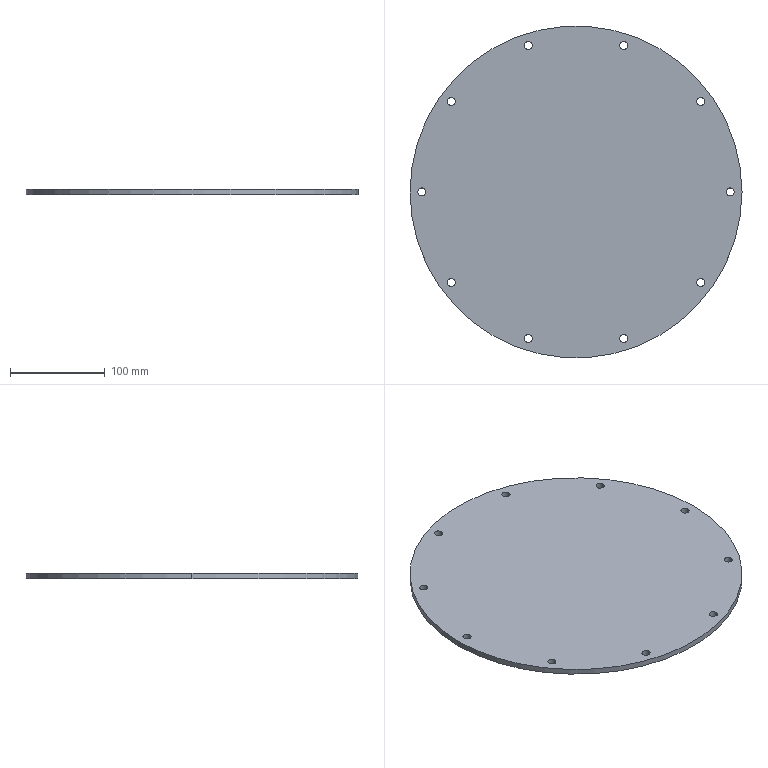Part | SolidWorks | features BaseBody 1 | 1 solid | 24 faces | box 350 x 350 x 6 mm | volume 573863 mm3 | cylinder 22 | plane 2 | commonest cylinder face diameters 8.5 x20 350 x2
STEP:
#1=CARTESIAN_POINT('',(127.215,95.515,-6.));
#2=VERTEX_POINT('',#1);
#3=CARTESIAN_POINT('',(135.715,95.515,-6.));
#4=VERTEX_POINT('',#3);
#5=CARTESIAN_POINT('',(131.465,95.515,-6.));
#6=DIRECTION('',(0.,0.,1.));
#7=DIRECTION('',(1.,0.,0.));
#8=AXIS2_PLACEMENT_3D('',#5,#6,#7);
#9=CIRCLE('',#8,4.25);
#10=EDGE_CURVE('',#2,#4,#9,.T.);
#11=ORIENTED_EDGE('',*,*,#10,.F.);
#12=CARTESIAN_POINT('',(127.215,95.515,0.));
#13=VERTEX_POINT('',#12);
#14=CARTESIAN_POINT('',(127.215,95.515,-20.));
#15=DIRECTION('',(0.,0.,1.));
#16=VECTOR('',#15,1000.);
#17=LINE('',#14,#16);
#18=EDGE_CURVE('',#2,#13,#17,.T.);
#19=ORIENTED_EDGE('',*,*,#18,.T.);
#20=CARTESIAN_POINT('',(135.715,95.515,0.));
#21=VERTEX_POINT('',#20);
#22=CARTESIAN_POINT('',(131.465,95.515,0.));
#23=DIRECTION('',(0.,0.,1.));
#24=DIRECTION('',(0.809,0.5878,0.));
#25=AXIS2_PLACEMENT_3D('',#22,#23,#24);
#26=CIRCLE('',#25,4.25);
#27=EDGE_CURVE('',#13,#21,#26,.T.);
#28=ORIENTED_EDGE('',*,*,#27,.T.);
#29=CARTESIAN_POINT('',(135.715,95.515,-20.));
#30=DIRECTION('',(0.,0.,1.));
#31=VECTOR('',#30,1000.);
#32=LINE('',#29,#31);
#33=EDGE_CURVE('',#4,#21,#32,.T.);
#34=ORIENTED_EDGE('',*,*,#33,.F.);
#35=EDGE_LOOP('',(#11,#19,#28,#34));
#36=FACE_OUTER_BOUND('',#35,.T.);
#37=CARTESIAN_POINT('',(131.465,95.515,-20.));
#38=DIRECTION('',(0.,0.,1.));
#39=DIRECTION('',(1.,0.,0.));
#40=AXIS2_PLACEMENT_3D('',#37,#38,#39);
#41=CYLINDRICAL_SURFACE('',#40,4.25);
#42=ADVANCED_FACE('',(#36),#41,.F.);
#43=CARTESIAN_POINT('',(45.965,154.547,-6.));
#44=VERTEX_POINT('',#43);
#45=CARTESIAN_POINT('',(54.465,154.547,-6.));
#46=VERTEX_POINT('',#45);
#47=CARTESIAN_POINT('',(50.215,154.547,-6.));
#48=DIRECTION('',(0.,0.,1.));
#49=DIRECTION('',(1.,0.,0.));
#50=AXIS2_PLACEMENT_3D('',#47,#48,#49);
#51=CIRCLE('',#50,4.25);
#52=EDGE_CURVE('',#44,#46,#51,.T.);
#53=ORIENTED_EDGE('',*,*,#52,.F.);
#54=CARTESIAN_POINT('',(45.965,154.547,0.));
#55=VERTEX_POINT('',#54);
#56=CARTESIAN_POINT('',(45.965,154.547,-20.));
#57=DIRECTION('',(0.,0.,1.));
#58=VECTOR('',#57,1000.);
#59=LINE('',#56,#58);
#60=EDGE_CURVE('',#44,#55,#59,.T.);
#61=ORIENTED_EDGE('',*,*,#60,.T.);
#62=CARTESIAN_POINT('',(54.465,154.547,0.));
#63=VERTEX_POINT('',#62);
#64=CARTESIAN_POINT('',(50.215,154.547,0.));
#65=DIRECTION('',(0.,0.,1.));
#66=DIRECTION('',(0.309,0.9511,0.));
#67=AXIS2_PLACEMENT_3D('',#64,#65,#66);
#68=CIRCLE('',#67,4.25);
#69=EDGE_CURVE('',#55,#63,#68,.T.);
#70=ORIENTED_EDGE('',*,*,#69,.T.);
#71=CARTESIAN_POINT('',(54.465,154.547,-20.));
#72=DIRECTION('',(0.,0.,1.));
#73=VECTOR('',#72,1000.);
#74=LINE('',#71,#73);
#75=EDGE_CURVE('',#46,#63,#74,.T.);
#76=ORIENTED_EDGE('',*,*,#75,.F.);
#77=EDGE_LOOP('',(#53,#61,#70,#76));
#78=FACE_OUTER_BOUND('',#77,.T.);
#79=CARTESIAN_POINT('',(50.215,154.547,-20.));
#80=DIRECTION('',(0.,0.,1.));
#81=DIRECTION('',(1.,0.,0.));
#82=AXIS2_PLACEMENT_3D('',#79,#80,#81);
#83=CYLINDRICAL_SURFACE('',#82,4.25);
#84=ADVANCED_FACE('',(#78),#83,.F.);
#85=CARTESIAN_POINT('',(-54.465,154.547,-6.));
#86=VERTEX_POINT('',#85);
#87=CARTESIAN_POINT('',(-45.965,154.547,-6.));
#88=VERTEX_POINT('',#87);
#89=CARTESIAN_POINT('',(-50.215,154.547,-6.));
#90=DIRECTION('',(0.,0.,1.));
#91=DIRECTION('',(1.,0.,0.));
#92=AXIS2_PLACEMENT_3D('',#89,#90,#91);
#93=CIRCLE('',#92,4.25);
#94=EDGE_CURVE('',#86,#88,#93,.T.);
#95=ORIENTED_EDGE('',*,*,#94,.F.);
#96=CARTESIAN_POINT('',(-54.465,154.547,0.));
#97=VERTEX_POINT('',#96);
#98=CARTESIAN_POINT('',(-54.465,154.547,-20.));
#99=DIRECTION('',(0.,0.,1.));
#100=VECTOR('',#99,1000.);
#101=LINE('',#98,#100);
#102=EDGE_CURVE('',#86,#97,#101,.T.);
#103=ORIENTED_EDGE('',*,*,#102,.T.);
#104=CARTESIAN_POINT('',(-45.965,154.547,0.));
#105=VERTEX_POINT('',#104);
#106=CARTESIAN_POINT('',(-50.215,154.547,0.));
#107=DIRECTION('',(0.,0.,1.));
#108=DIRECTION('',(-0.309,0.9511,0.));
#109=AXIS2_PLACEMENT_3D('',#106,#107,#108);
#110=CIRCLE('',#109,4.25);
#111=EDGE_CURVE('',#97,#105,#110,.T.);
#112=ORIENTED_EDGE('',*,*,#111,.T.);
#113=CARTESIAN_POINT('',(-45.965,154.547,-20.));
#114=DIRECTION('',(0.,0.,1.));
#115=VECTOR('',#114,1000.);
#116=LINE('',#113,#115);
#117=EDGE_CURVE('',#88,#105,#116,.T.);
#118=ORIENTED_EDGE('',*,*,#117,.F.);
#119=EDGE_LOOP('',(#95,#103,#112,#118));
#120=FACE_OUTER_BOUND('',#119,.T.);
#121=CARTESIAN_POINT('',(-50.215,154.547,-20.));
#122=DIRECTION('',(0.,0.,1.));
#123=DIRECTION('',(1.,0.,0.));
#124=AXIS2_PLACEMENT_3D('',#121,#122,#123);
#125=CYLINDRICAL_SURFACE('',#124,4.25);
#126=ADVANCED_FACE('',(#120),#125,.F.);
#127=CARTESIAN_POINT('',(-135.715,95.515,-6.));
#128=VERTEX_POINT('',#127);
#129=CARTESIAN_POINT('',(-127.215,95.515,-6.));
#130=VERTEX_POINT('',#129);
#131=CARTESIAN_POINT('',(-131.465,95.515,-6.));
#132=DIRECTION('',(0.,0.,1.));
#133=DIRECTION('',(1.,0.,0.));
#134=AXIS2_PLACEMENT_3D('',#131,#132,#133);
#135=CIRCLE('',#134,4.25);
#136=EDGE_CURVE('',#128,#130,#135,.T.);
#137=ORIENTED_EDGE('',*,*,#136,.F.);
#138=CARTESIAN_POINT('',(-135.715,95.515,0.));
#139=VERTEX_POINT('',#138);
#140=CARTESIAN_POINT('',(-135.715,95.515,-20.));
#141=DIRECTION('',(0.,0.,1.));
#142=VECTOR('',#141,1000.);
#143=LINE('',#140,#142);
#144=EDGE_CURVE('',#128,#139,#143,.T.);
#145=ORIENTED_EDGE('',*,*,#144,.T.);
#146=CARTESIAN_POINT('',(-127.215,95.515,0.));
#147=VERTEX_POINT('',#146);
#148=CARTESIAN_POINT('',(-131.465,95.515,0.));
#149=DIRECTION('',(0.,0.,1.));
#150=DIRECTION('',(-0.809,0.5878,0.));
#151=AXIS2_PLACEMENT_3D('',#148,#149,#150);
#152=CIRCLE('',#151,4.25);
#153=EDGE_CURVE('',#139,#147,#152,.T.);
#154=ORIENTED_EDGE('',*,*,#153,.T.);
#155=CARTESIAN_POINT('',(-127.215,95.515,-20.));
#156=DIRECTION('',(0.,0.,1.));
#157=VECTOR('',#156,1000.);
#158=LINE('',#155,#157);
#159=EDGE_CURVE('',#130,#147,#158,.T.);
#160=ORIENTED_EDGE('',*,*,#159,.F.);
#161=EDGE_LOOP('',(#137,#145,#154,#160));
#162=FACE_OUTER_BOUND('',#161,.T.);
#163=CARTESIAN_POINT('',(-131.465,95.515,-20.));
#164=DIRECTION('',(0.,0.,1.));
#165=DIRECTION('',(1.,0.,0.));
#166=AXIS2_PLACEMENT_3D('',#163,#164,#165);
#167=CYLINDRICAL_SURFACE('',#166,4.25);
#168=ADVANCED_FACE('',(#162),#167,.F.);
#169=CARTESIAN_POINT('',(-166.75,0.,-6.));
#170=VERTEX_POINT('',#169);
#171=CARTESIAN_POINT('',(-158.25,0.,-6.));
#172=VERTEX_POINT('',#171);
#173=CARTESIAN_POINT('',(-162.5,0.,-6.));
#174=DIRECTION('',(0.,0.,1.));
#175=DIRECTION('',(1.,0.,0.));
#176=AXIS2_PLACEMENT_3D('',#173,#174,#175);
#177=CIRCLE('',#176,4.25);
#178=EDGE_CURVE('',#170,#172,#177,.T.);
#179=ORIENTED_EDGE('',*,*,#178,.F.);
#180=CARTESIAN_POINT('',(-166.75,0.,0.));
#181=VERTEX_POINT('',#180);
#182=CARTESIAN_POINT('',(-166.75,0.,-20.));
#183=DIRECTION('',(0.,0.,1.));
#184=VECTOR('',#183,1000.);
#185=LINE('',#182,#184);
#186=EDGE_CURVE('',#170,#181,#185,.T.);
#187=ORIENTED_EDGE('',*,*,#186,.T.);
#188=CARTESIAN_POINT('',(-158.25,0.,0.));
#189=VERTEX_POINT('',#188);
#190=CARTESIAN_POINT('',(-162.5,0.,0.));
#191=DIRECTION('',(0.,0.,1.));
#192=DIRECTION('',(-1.,0.,0.));
#193=AXIS2_PLACEMENT_3D('',#190,#191,#192);
#194=CIRCLE('',#193,4.25);
#195=EDGE_CURVE('',#181,#189,#194,.T.);
#196=ORIENTED_EDGE('',*,*,#195,.T.);
#197=CARTESIAN_POINT('',(-158.25,0.,-20.));
#198=DIRECTION('',(0.,0.,1.));
#199=VECTOR('',#198,1000.);
#200=LINE('',#197,#199);
#201=EDGE_CURVE('',#172,#189,#200,.T.);
#202=ORIENTED_EDGE('',*,*,#201,.F.);
#203=EDGE_LOOP('',(#179,#187,#196,#202));
#204=FACE_OUTER_BOUND('',#203,.T.);
#205=CARTESIAN_POINT('',(-162.5,0.,-20.));
#206=DIRECTION('',(0.,0.,1.));
#207=DIRECTION('',(1.,0.,0.));
#208=AXIS2_PLACEMENT_3D('',#205,#206,#207);
#209=CYLINDRICAL_SURFACE('',#208,4.25);
#210=ADVANCED_FACE('',(#204),#209,.F.);
#211=CARTESIAN_POINT('',(-135.715,-95.515,-6.));
#212=VERTEX_POINT('',#211);
#213=CARTESIAN_POINT('',(-127.215,-95.515,-6.));
#214=VERTEX_POINT('',#213);
#215=CARTESIAN_POINT('',(-131.465,-95.515,-6.));
#216=DIRECTION('',(0.,0.,1.));
#217=DIRECTION('',(1.,0.,0.));
#218=AXIS2_PLACEMENT_3D('',#215,#216,#217);
#219=CIRCLE('',#218,4.25);
#220=EDGE_CURVE('',#212,#214,#219,.T.);
#221=ORIENTED_EDGE('',*,*,#220,.F.);
#222=CARTESIAN_POINT('',(-135.715,-95.515,0.));
#223=VERTEX_POINT('',#222);
#224=CARTESIAN_POINT('',(-135.715,-95.515,-20.));
#225=DIRECTION('',(0.,0.,1.));
#226=VECTOR('',#225,1000.);
#227=LINE('',#224,#226);
#228=EDGE_CURVE('',#212,#223,#227,.T.);
#229=ORIENTED_EDGE('',*,*,#228,.T.);
#230=CARTESIAN_POINT('',(-127.215,-95.515,0.));
#231=VERTEX_POINT('',#230);
#232=CARTESIAN_POINT('',(-131.465,-95.515,0.));
#233=DIRECTION('',(0.,0.,1.));
#234=DIRECTION('',(-0.809,-0.5878,0.));
#235=AXIS2_PLACEMENT_3D('',#232,#233,#234);
#236=CIRCLE('',#235,4.25);
#237=EDGE_CURVE('',#223,#231,#236,.T.);
#238=ORIENTED_EDGE('',*,*,#237,.T.);
#239=CARTESIAN_POINT('',(-127.215,-95.515,-20.));
#240=DIRECTION('',(0.,0.,1.));
#241=VECTOR('',#240,1000.);
#242=LINE('',#239,#241);
#243=EDGE_CURVE('',#214,#231,#242,.T.);
#244=ORIENTED_EDGE('',*,*,#243,.F.);
#245=EDGE_LOOP('',(#221,#229,#238,#244));
#246=FACE_OUTER_BOUND('',#245,.T.);
#247=CARTESIAN_POINT('',(-131.465,-95.515,-20.));
#248=DIRECTION('',(0.,0.,1.));
#249=DIRECTION('',(1.,0.,0.));
#250=AXIS2_PLACEMENT_3D('',#247,#248,#249);
#251=CYLINDRICAL_SURFACE('',#250,4.25);
#252=ADVANCED_FACE('',(#246),#251,.F.);
#253=CARTESIAN_POINT('',(-54.465,-154.547,-6.));
#254=VERTEX_POINT('',#253);
#255=CARTESIAN_POINT('',(-45.965,-154.547,-6.));
#256=VERTEX_POINT('',#255);
#257=CARTESIAN_POINT('',(-50.215,-154.547,-6.));
#258=DIRECTION('',(0.,0.,1.));
#259=DIRECTION('',(1.,0.,0.));
#260=AXIS2_PLACEMENT_3D('',#257,#258,#259);
#261=CIRCLE('',#260,4.25);
#262=EDGE_CURVE('',#254,#256,#261,.T.);
#263=ORIENTED_EDGE('',*,*,#262,.F.);
#264=CARTESIAN_POINT('',(-54.465,-154.547,0.));
#265=VERTEX_POINT('',#264);
#266=CARTESIAN_POINT('',(-54.465,-154.547,-20.));
#267=DIRECTION('',(0.,0.,1.));
#268=VECTOR('',#267,1000.);
#269=LINE('',#266,#268);
#270=EDGE_CURVE('',#254,#265,#269,.T.);
#271=ORIENTED_EDGE('',*,*,#270,.T.);
#272=CARTESIAN_POINT('',(-45.965,-154.547,0.));
#273=VERTEX_POINT('',#272);
#274=CARTESIAN_POINT('',(-50.215,-154.547,0.));
#275=DIRECTION('',(0.,0.,1.));
#276=DIRECTION('',(-0.309,-0.9511,0.));
#277=AXIS2_PLACEMENT_3D('',#274,#275,#276);
#278=CIRCLE('',#277,4.25);
#279=EDGE_CURVE('',#265,#273,#278,.T.);
#280=ORIENTED_EDGE('',*,*,#279,.T.);
#281=CARTESIAN_POINT('',(-45.965,-154.547,-20.));
#282=DIRECTION('',(0.,0.,1.));
#283=VECTOR('',#282,1000.);
#284=LINE('',#281,#283);
#285=EDGE_CURVE('',#256,#273,#284,.T.);
#286=ORIENTED_EDGE('',*,*,#285,.F.);
#287=EDGE_LOOP('',(#263,#271,#280,#286));
#288=FACE_OUTER_BOUND('',#287,.T.);
#289=CARTESIAN_POINT('',(-50.215,-154.547,-20.));
#290=DIRECTION('',(0.,0.,1.));
#291=DIRECTION('',(1.,0.,0.));
#292=AXIS2_PLACEMENT_3D('',#289,#290,#291);
#293=CYLINDRICAL_SURFACE('',#292,4.25);
#294=ADVANCED_FACE('',(#288),#293,.F.);
#295=CARTESIAN_POINT('',(45.965,-154.547,-6.));
#296=VERTEX_POINT('',#295);
#297=CARTESIAN_POINT('',(54.465,-154.547,-6.));
#298=VERTEX_POINT('',#297);
#299=CARTESIAN_POINT('',(50.215,-154.547,-6.));
#300=DIRECTION('',(0.,0.,1.));
#301=DIRECTION('',(1.,0.,0.));
#302=AXIS2_PLACEMENT_3D('',#299,#300,#301);
#303=CIRCLE('',#302,4.25);
#304=EDGE_CURVE('',#296,#298,#303,.T.);
#305=ORIENTED_EDGE('',*,*,#304,.F.);
#306=CARTESIAN_POINT('',(45.965,-154.547,0.));
#307=VERTEX_POINT('',#306);
#308=CARTESIAN_POINT('',(45.965,-154.547,-20.));
#309=DIRECTION('',(0.,0.,1.));
#310=VECTOR('',#309,1000.);
#311=LINE('',#308,#310);
#312=EDGE_CURVE('',#296,#307,#311,.T.);
#313=ORIENTED_EDGE('',*,*,#312,.T.);
#314=CARTESIAN_POINT('',(54.465,-154.547,0.));
#315=VERTEX_POINT('',#314);
#316=CARTESIAN_POINT('',(50.215,-154.547,0.));
#317=DIRECTION('',(0.,0.,1.));
#318=DIRECTION('',(0.309,-0.9511,0.));
#319=AXIS2_PLACEMENT_3D('',#316,#317,#318);
#320=CIRCLE('',#319,4.25);
#321=EDGE_CURVE('',#307,#315,#320,.T.);
#322=ORIENTED_EDGE('',*,*,#321,.T.);
#323=CARTESIAN_POINT('',(54.465,-154.547,-20.));
#324=DIRECTION('',(0.,0.,1.));
#325=VECTOR('',#324,1000.);
#326=LINE('',#323,#325);
#327=EDGE_CURVE('',#298,#315,#326,.T.);
#328=ORIENTED_EDGE('',*,*,#327,.F.);
#329=EDGE_LOOP('',(#305,#313,#322,#328));
#330=FACE_OUTER_BOUND('',#329,.T.);
#331=CARTESIAN_POINT('',(50.215,-154.547,-20.));
#332=DIRECTION('',(0.,0.,1.));
#333=DIRECTION('',(1.,0.,0.));
#334=AXIS2_PLACEMENT_3D('',#331,#332,#333);
#335=CYLINDRICAL_SURFACE('',#334,4.25);
#336=ADVANCED_FACE('',(#330),#335,.F.);
#337=CARTESIAN_POINT('',(127.215,-95.515,-6.));
#338=VERTEX_POINT('',#337);
#339=CARTESIAN_POINT('',(135.715,-95.515,-6.));
#340=VERTEX_POINT('',#339);
#341=CARTESIAN_POINT('',(131.465,-95.515,-6.));
#342=DIRECTION('',(0.,0.,1.));
#343=DIRECTION('',(1.,0.,0.));
#344=AXIS2_PLACEMENT_3D('',#341,#342,#343);
#345=CIRCLE('',#344,4.25);
#346=EDGE_CURVE('',#338,#340,#345,.T.);
#347=ORIENTED_EDGE('',*,*,#346,.F.);
#348=CARTESIAN_POINT('',(127.215,-95.515,0.));
#349=VERTEX_POINT('',#348);
#350=CARTESIAN_POINT('',(127.215,-95.515,-20.));
#351=DIRECTION('',(0.,0.,1.));
#352=VECTOR('',#351,1000.);
#353=LINE('',#350,#352);
#354=EDGE_CURVE('',#338,#349,#353,.T.);
#355=ORIENTED_EDGE('',*,*,#354,.T.);
#356=CARTESIAN_POINT('',(135.715,-95.515,0.));
#357=VERTEX_POINT('',#356);
#358=CARTESIAN_POINT('',(131.465,-95.515,0.));
#359=DIRECTION('',(0.,0.,1.));
#360=DIRECTION('',(0.809,-0.5878,0.));
#361=AXIS2_PLACEMENT_3D('',#358,#359,#360);
#362=CIRCLE('',#361,4.25);
#363=EDGE_CURVE('',#349,#357,#362,.T.);
#364=ORIENTED_EDGE('',*,*,#363,.T.);
#365=CARTESIAN_POINT('',(135.715,-95.515,-20.));
#366=DIRECTION('',(0.,0.,1.));
#367=VECTOR('',#366,1000.);
#368=LINE('',#365,#367);
#369=EDGE_CURVE('',#340,#357,#368,.T.);
#370=ORIENTED_EDGE('',*,*,#369,.F.);
#371=EDGE_LOOP('',(#347,#355,#364,#370));
#372=FACE_OUTER_BOUND('',#371,.T.);
#373=CARTESIAN_POINT('',(131.465,-95.515,-20.));
#374=DIRECTION('',(0.,0.,1.));
#375=DIRECTION('',(1.,0.,0.));
#376=AXIS2_PLACEMENT_3D('',#373,#374,#375);
#377=CYLINDRICAL_SURFACE('',#376,4.25);
#378=ADVANCED_FACE('',(#372),#377,.F.);
#379=CARTESIAN_POINT('',(158.25,0.,-6.));
#380=VERTEX_POINT('',#379);
#381=CARTESIAN_POINT('',(166.75,0.,-6.));
#382=VERTEX_POINT('',#381);
#383=CARTESIAN_POINT('',(162.5,0.,-6.));
#384=DIRECTION('',(0.,0.,1.));
#385=DIRECTION('',(1.,0.,0.));
#386=AXIS2_PLACEMENT_3D('',#383,#384,#385);
#387=CIRCLE('',#386,4.25);
#388=EDGE_CURVE('',#380,#382,#387,.T.);
#389=ORIENTED_EDGE('',*,*,#388,.F.);
#390=CARTESIAN_POINT('',(158.25,0.,0.));
#391=VERTEX_POINT('',#390);
#392=CARTESIAN_POINT('',(158.25,0.,-20.));
#393=DIRECTION('',(0.,0.,1.));
#394=VECTOR('',#393,1000.);
#395=LINE('',#392,#394);
#396=EDGE_CURVE('',#380,#391,#395,.T.);
#397=ORIENTED_EDGE('',*,*,#396,.T.);
#398=CARTESIAN_POINT('',(166.75,0.,0.));
#399=VERTEX_POINT('',#398);
#400=CARTESIAN_POINT('',(162.5,0.,0.));
#401=DIRECTION('',(0.,0.,1.));
#402=DIRECTION('',(1.,0.,0.));
#403=AXIS2_PLACEMENT_3D('',#400,#401,#402);
#404=CIRCLE('',#403,4.25);
#405=EDGE_CURVE('',#391,#399,#404,.T.);
#406=ORIENTED_EDGE('',*,*,#405,.T.);
#407=CARTESIAN_POINT('',(166.75,0.,-20.));
#408=DIRECTION('',(0.,0.,1.));
#409=VECTOR('',#408,1000.);
#410=LINE('',#407,#409);
#411=EDGE_CURVE('',#382,#399,#410,.T.);
#412=ORIENTED_EDGE('',*,*,#411,.F.);
#413=EDGE_LOOP('',(#389,#397,#406,#412));
#414=FACE_OUTER_BOUND('',#413,.T.);
#415=CARTESIAN_POINT('',(162.5,0.,-20.));
#416=DIRECTION('',(0.,0.,1.));
#417=DIRECTION('',(1.,0.,0.));
#418=AXIS2_PLACEMENT_3D('',#415,#416,#417);
#419=CYLINDRICAL_SURFACE('',#418,4.25);
#420=ADVANCED_FACE('',(#414),#419,.F.);
#421=CARTESIAN_POINT('',(175.,0.,-6.));
#422=VERTEX_POINT('',#421);
#423=CARTESIAN_POINT('',(-175.,0.,-6.));
#424=VERTEX_POINT('',#423);
#425=CARTESIAN_POINT('',(0.,0.,-6.));
#426=DIRECTION('',(0.,0.,1.));
#427=DIRECTION('',(1.,0.,0.));
#428=AXIS2_PLACEMENT_3D('',#425,#426,#427);
#429=CIRCLE('',#428,175.);
#430=EDGE_CURVE('',#422,#424,#429,.T.);
#431=ORIENTED_EDGE('',*,*,#430,.T.);
#432=CARTESIAN_POINT('',(-175.,0.,0.));
#433=VERTEX_POINT('',#432);
#434=CARTESIAN_POINT('',(-175.,0.,-6.));
#435=DIRECTION('',(0.,0.,1.));
#436=VECTOR('',#435,1000.);
#437=LINE('',#434,#436);
#438=EDGE_CURVE('',#424,#433,#437,.T.);
#439=ORIENTED_EDGE('',*,*,#438,.T.);
#440=CARTESIAN_POINT('',(175.,0.,0.));
#441=VERTEX_POINT('',#440);
#442=CARTESIAN_POINT('',(0.,0.,0.));
#443=DIRECTION('',(0.,0.,1.));
#444=DIRECTION('',(1.,0.,0.));
#445=AXIS2_PLACEMENT_3D('',#442,#443,#444);
#446=CIRCLE('',#445,175.);
#447=EDGE_CURVE('',#441,#433,#446,.T.);
#448=ORIENTED_EDGE('',*,*,#447,.F.);
#449=CARTESIAN_POINT('',(175.,0.,-6.));
#450=DIRECTION('',(0.,0.,1.));
#451=VECTOR('',#450,1000.);
#452=LINE('',#449,#451);
#453=EDGE_CURVE('',#422,#441,#452,.T.);
#454=ORIENTED_EDGE('',*,*,#453,.F.);
#455=EDGE_LOOP('',(#431,#439,#448,#454));
#456=FACE_OUTER_BOUND('',#455,.T.);
#457=CARTESIAN_POINT('',(0.,0.,-6.));
#458=DIRECTION('',(0.,0.,1.));
#459=DIRECTION('',(1.,0.,0.));
#460=AXIS2_PLACEMENT_3D('',#457,#458,#459);
#461=CYLINDRICAL_SURFACE('',#460,175.);
#462=ADVANCED_FACE('',(#456),#461,.T.);
#463=ORIENTED_EDGE('',*,*,#438,.F.);
#464=CARTESIAN_POINT('',(0.,0.,-6.));
#465=DIRECTION('',(0.,0.,1.));
#466=DIRECTION('',(1.,0.,0.));
#467=AXIS2_PLACEMENT_3D('',#464,#465,#466);
#468=CIRCLE('',#467,175.);
#469=EDGE_CURVE('',#424,#422,#468,.T.);
#470=ORIENTED_EDGE('',*,*,#469,.T.);
#471=ORIENTED_EDGE('',*,*,#453,.T.);
#472=CARTESIAN_POINT('',(0.,0.,0.));
#473=DIRECTION('',(0.,0.,1.));
#474=DIRECTION('',(1.,0.,0.));
#475=AXIS2_PLACEMENT_3D('',#472,#473,#474);
#476=CIRCLE('',#475,175.);
#477=EDGE_CURVE('',#433,#441,#476,.T.);
#478=ORIENTED_EDGE('',*,*,#477,.F.);
#479=EDGE_LOOP('',(#463,#470,#471,#478));
#480=FACE_OUTER_BOUND('',#479,.T.);
#481=CARTESIAN_POINT('',(0.,0.,-6.));
#482=DIRECTION('',(0.,0.,1.));
#483=DIRECTION('',(1.,0.,0.));
#484=AXIS2_PLACEMENT_3D('',#481,#482,#483);
#485=CYLINDRICAL_SURFACE('',#484,175.);
#486=ADVANCED_FACE('',(#480),#485,.T.);
#487=ORIENTED_EDGE('',*,*,#430,.F.);
#488=ORIENTED_EDGE('',*,*,#469,.F.);
#489=EDGE_LOOP('',(#487,#488));
#490=FACE_OUTER_BOUND('',#489,.T.);
#491=CARTESIAN_POINT('',(131.465,95.515,-6.));
#492=DIRECTION('',(0.,0.,1.));
#493=DIRECTION('',(1.,0.,0.));
#494=AXIS2_PLACEMENT_3D('',#491,#492,#493);
#495=CIRCLE('',#494,4.25);
#496=EDGE_CURVE('',#4,#2,#495,.T.);
#497=ORIENTED_EDGE('',*,*,#496,.T.);
#498=ORIENTED_EDGE('',*,*,#10,.T.);
#499=EDGE_LOOP('',(#497,#498));
#500=FACE_BOUND('',#499,.T.);
#501=CARTESIAN_POINT('',(50.215,154.547,-6.));
#502=DIRECTION('',(0.,0.,1.));
#503=DIRECTION('',(1.,0.,0.));
#504=AXIS2_PLACEMENT_3D('',#501,#502,#503);
#505=CIRCLE('',#504,4.25);
#506=EDGE_CURVE('',#46,#44,#505,.T.);
#507=ORIENTED_EDGE('',*,*,#506,.T.);
#508=ORIENTED_EDGE('',*,*,#52,.T.);
#509=EDGE_LOOP('',(#507,#508));
#510=FACE_BOUND('',#509,.T.);
#511=CARTESIAN_POINT('',(-50.215,154.547,-6.));
#512=DIRECTION('',(0.,0.,1.));
#513=DIRECTION('',(1.,0.,0.));
#514=AXIS2_PLACEMENT_3D('',#511,#512,#513);
#515=CIRCLE('',#514,4.25);
#516=EDGE_CURVE('',#88,#86,#515,.T.);
#517=ORIENTED_EDGE('',*,*,#516,.T.);
#518=ORIENTED_EDGE('',*,*,#94,.T.);
#519=EDGE_LOOP('',(#517,#518));
#520=FACE_BOUND('',#519,.T.);
#521=CARTESIAN_POINT('',(-131.465,95.515,-6.));
#522=DIRECTION('',(0.,0.,1.));
#523=DIRECTION('',(1.,0.,0.));
#524=AXIS2_PLACEMENT_3D('',#521,#522,#523);
#525=CIRCLE('',#524,4.25);
#526=EDGE_CURVE('',#130,#128,#525,.T.);
#527=ORIENTED_EDGE('',*,*,#526,.T.);
#528=ORIENTED_EDGE('',*,*,#136,.T.);
#529=EDGE_LOOP('',(#527,#528));
#530=FACE_BOUND('',#529,.T.);
#531=CARTESIAN_POINT('',(-162.5,0.,-6.));
#532=DIRECTION('',(0.,0.,1.));
#533=DIRECTION('',(1.,0.,0.));
#534=AXIS2_PLACEMENT_3D('',#531,#532,#533);
#535=CIRCLE('',#534,4.25);
#536=EDGE_CURVE('',#172,#170,#535,.T.);
#537=ORIENTED_EDGE('',*,*,#536,.T.);
#538=ORIENTED_EDGE('',*,*,#178,.T.);
#539=EDGE_LOOP('',(#537,#538));
#540=FACE_BOUND('',#539,.T.);
#541=CARTESIAN_POINT('',(-131.465,-95.515,-6.));
#542=DIRECTION('',(0.,0.,1.));
#543=DIRECTION('',(1.,0.,0.));
#544=AXIS2_PLACEMENT_3D('',#541,#542,#543);
#545=CIRCLE('',#544,4.25);
#546=EDGE_CURVE('',#214,#212,#545,.T.);
#547=ORIENTED_EDGE('',*,*,#546,.T.);
#548=ORIENTED_EDGE('',*,*,#220,.T.);
#549=EDGE_LOOP('',(#547,#548));
#550=FACE_BOUND('',#549,.T.);
#551=CARTESIAN_POINT('',(-50.215,-154.547,-6.));
#552=DIRECTION('',(0.,0.,1.));
#553=DIRECTION('',(1.,0.,0.));
#554=AXIS2_PLACEMENT_3D('',#551,#552,#553);
#555=CIRCLE('',#554,4.25);
#556=EDGE_CURVE('',#256,#254,#555,.T.);
#557=ORIENTED_EDGE('',*,*,#556,.T.);
#558=ORIENTED_EDGE('',*,*,#262,.T.);
#559=EDGE_LOOP('',(#557,#558));
#560=FACE_BOUND('',#559,.T.);
#561=CARTESIAN_POINT('',(50.215,-154.547,-6.));
#562=DIRECTION('',(0.,0.,1.));
#563=DIRECTION('',(1.,0.,0.));
#564=AXIS2_PLACEMENT_3D('',#561,#562,#563);
#565=CIRCLE('',#564,4.25);
#566=EDGE_CURVE('',#298,#296,#565,.T.);
#567=ORIENTED_EDGE('',*,*,#566,.T.);
#568=ORIENTED_EDGE('',*,*,#304,.T.);
#569=EDGE_LOOP('',(#567,#568));
#570=FACE_BOUND('',#569,.T.);
#571=CARTESIAN_POINT('',(131.465,-95.515,-6.));
#572=DIRECTION('',(0.,0.,1.));
#573=DIRECTION('',(1.,0.,0.));
#574=AXIS2_PLACEMENT_3D('',#571,#572,#573);
#575=CIRCLE('',#574,4.25);
#576=EDGE_CURVE('',#340,#338,#575,.T.);
#577=ORIENTED_EDGE('',*,*,#576,.T.);
#578=ORIENTED_EDGE('',*,*,#346,.T.);
#579=EDGE_LOOP('',(#577,#578));
#580=FACE_BOUND('',#579,.T.);
#581=CARTESIAN_POINT('',(162.5,0.,-6.));
#582=DIRECTION('',(0.,0.,1.));
#583=DIRECTION('',(1.,0.,0.));
#584=AXIS2_PLACEMENT_3D('',#581,#582,#583);
#585=CIRCLE('',#584,4.25);
#586=EDGE_CURVE('',#382,#380,#585,.T.);
#587=ORIENTED_EDGE('',*,*,#586,.T.);
#588=ORIENTED_EDGE('',*,*,#388,.T.);
#589=EDGE_LOOP('',(#587,#588));
#590=FACE_BOUND('',#589,.T.);
#591=CARTESIAN_POINT('',(0.,0.,-6.));
#592=DIRECTION('',(0.,0.,1.));
#593=DIRECTION('',(1.,0.,0.));
#594=AXIS2_PLACEMENT_3D('',#591,#592,#593);
#595=PLANE('',#594);
#596=ADVANCED_FACE('',(#490,#500,#510,#520,#530,#540,#550,#560,#570,#580,#590),#595,.F.);
#597=ORIENTED_EDGE('',*,*,#447,.T.);
#598=ORIENTED_EDGE('',*,*,#477,.T.);
#599=EDGE_LOOP('',(#597,#598));
#600=FACE_OUTER_BOUND('',#599,.T.);
#601=CARTESIAN_POINT('',(131.465,95.515,0.));
#602=DIRECTION('',(0.,0.,1.));
#603=DIRECTION('',(0.809,0.5878,0.));
#604=AXIS2_PLACEMENT_3D('',#601,#602,#603);
#605=CIRCLE('',#604,4.25);
#606=EDGE_CURVE('',#21,#13,#605,.T.);
#607=ORIENTED_EDGE('',*,*,#606,.F.);
#608=ORIENTED_EDGE('',*,*,#27,.F.);
#609=EDGE_LOOP('',(#607,#608));
#610=FACE_BOUND('',#609,.T.);
#611=CARTESIAN_POINT('',(50.215,154.547,0.));
#612=DIRECTION('',(0.,0.,1.));
#613=DIRECTION('',(0.309,0.9511,0.));
#614=AXIS2_PLACEMENT_3D('',#611,#612,#613);
#615=CIRCLE('',#614,4.25);
#616=EDGE_CURVE('',#63,#55,#615,.T.);
#617=ORIENTED_EDGE('',*,*,#616,.F.);
#618=ORIENTED_EDGE('',*,*,#69,.F.);
#619=EDGE_LOOP('',(#617,#618));
#620=FACE_BOUND('',#619,.T.);
#621=CARTESIAN_POINT('',(-50.215,154.547,0.));
#622=DIRECTION('',(0.,0.,1.));
#623=DIRECTION('',(-0.309,0.9511,0.));
#624=AXIS2_PLACEMENT_3D('',#621,#622,#623);
#625=CIRCLE('',#624,4.25);
#626=EDGE_CURVE('',#105,#97,#625,.T.);
#627=ORIENTED_EDGE('',*,*,#626,.F.);
#628=ORIENTED_EDGE('',*,*,#111,.F.);
#629=EDGE_LOOP('',(#627,#628));
#630=FACE_BOUND('',#629,.T.);
#631=CARTESIAN_POINT('',(-131.465,95.515,0.));
#632=DIRECTION('',(0.,0.,1.));
#633=DIRECTION('',(-0.809,0.5878,0.));
#634=AXIS2_PLACEMENT_3D('',#631,#632,#633);
#635=CIRCLE('',#634,4.25);
#636=EDGE_CURVE('',#147,#139,#635,.T.);
#637=ORIENTED_EDGE('',*,*,#636,.F.);
#638=ORIENTED_EDGE('',*,*,#153,.F.);
#639=EDGE_LOOP('',(#637,#638));
#640=FACE_BOUND('',#639,.T.);
#641=CARTESIAN_POINT('',(-162.5,0.,0.));
#642=DIRECTION('',(0.,0.,1.));
#643=DIRECTION('',(-1.,0.,0.));
#644=AXIS2_PLACEMENT_3D('',#641,#642,#643);
#645=CIRCLE('',#644,4.25);
#646=EDGE_CURVE('',#189,#181,#645,.T.);
#647=ORIENTED_EDGE('',*,*,#646,.F.);
#648=ORIENTED_EDGE('',*,*,#195,.F.);
#649=EDGE_LOOP('',(#647,#648));
#650=FACE_BOUND('',#649,.T.);
#651=CARTESIAN_POINT('',(-131.465,-95.515,0.));
#652=DIRECTION('',(0.,0.,1.));
#653=DIRECTION('',(-0.809,-0.5878,0.));
#654=AXIS2_PLACEMENT_3D('',#651,#652,#653);
#655=CIRCLE('',#654,4.25);
#656=EDGE_CURVE('',#231,#223,#655,.T.);
#657=ORIENTED_EDGE('',*,*,#656,.F.);
#658=ORIENTED_EDGE('',*,*,#237,.F.);
#659=EDGE_LOOP('',(#657,#658));
#660=FACE_BOUND('',#659,.T.);
#661=CARTESIAN_POINT('',(-50.215,-154.547,0.));
#662=DIRECTION('',(0.,0.,1.));
#663=DIRECTION('',(-0.309,-0.9511,0.));
#664=AXIS2_PLACEMENT_3D('',#661,#662,#663);
#665=CIRCLE('',#664,4.25);
#666=EDGE_CURVE('',#273,#265,#665,.T.);
#667=ORIENTED_EDGE('',*,*,#666,.F.);
#668=ORIENTED_EDGE('',*,*,#279,.F.);
#669=EDGE_LOOP('',(#667,#668));
#670=FACE_BOUND('',#669,.T.);
#671=CARTESIAN_POINT('',(50.215,-154.547,0.));
#672=DIRECTION('',(0.,0.,1.));
#673=DIRECTION('',(0.309,-0.9511,0.));
#674=AXIS2_PLACEMENT_3D('',#671,#672,#673);
#675=CIRCLE('',#674,4.25);
#676=EDGE_CURVE('',#315,#307,#675,.T.);
#677=ORIENTED_EDGE('',*,*,#676,.F.);
#678=ORIENTED_EDGE('',*,*,#321,.F.);
#679=EDGE_LOOP('',(#677,#678));
#680=FACE_BOUND('',#679,.T.);
#681=CARTESIAN_POINT('',(131.465,-95.515,0.));
#682=DIRECTION('',(0.,0.,1.));
#683=DIRECTION('',(0.809,-0.5878,0.));
#684=AXIS2_PLACEMENT_3D('',#681,#682,#683);
#685=CIRCLE('',#684,4.25);
#686=EDGE_CURVE('',#357,#349,#685,.T.);
#687=ORIENTED_EDGE('',*,*,#686,.F.);
#688=ORIENTED_EDGE('',*,*,#363,.F.);
#689=EDGE_LOOP('',(#687,#688));
#690=FACE_BOUND('',#689,.T.);
#691=CARTESIAN_POINT('',(162.5,0.,0.));
#692=DIRECTION('',(0.,0.,1.));
#693=DIRECTION('',(1.,0.,0.));
#694=AXIS2_PLACEMENT_3D('',#691,#692,#693);
#695=CIRCLE('',#694,4.25);
#696=EDGE_CURVE('',#399,#391,#695,.T.);
#697=ORIENTED_EDGE('',*,*,#696,.F.);
#698=ORIENTED_EDGE('',*,*,#405,.F.);
#699=EDGE_LOOP('',(#697,#698));
#700=FACE_BOUND('',#699,.T.);
#701=CARTESIAN_POINT('',(0.,0.,0.));
#702=DIRECTION('',(0.,0.,1.));
#703=DIRECTION('',(1.,0.,0.));
#704=AXIS2_PLACEMENT_3D('',#701,#702,#703);
#705=PLANE('',#704);
#706=ADVANCED_FACE('',(#600,#610,#620,#630,#640,#650,#660,#670,#680,#690,#700),#705,.T.);
#707=ORIENTED_EDGE('',*,*,#396,.F.);
#708=ORIENTED_EDGE('',*,*,#586,.F.);
#709=ORIENTED_EDGE('',*,*,#411,.T.);
#710=ORIENTED_EDGE('',*,*,#696,.T.);
#711=EDGE_LOOP('',(#707,#708,#709,#710));
#712=FACE_OUTER_BOUND('',#711,.T.);
#713=CARTESIAN_POINT('',(162.5,0.,-20.));
#714=DIRECTION('',(0.,0.,1.));
#715=DIRECTION('',(1.,0.,0.));
#716=AXIS2_PLACEMENT_3D('',#713,#714,#715);
#717=CYLINDRICAL_SURFACE('',#716,4.25);
#718=ADVANCED_FACE('',(#712),#717,.F.);
#719=ORIENTED_EDGE('',*,*,#354,.F.);
#720=ORIENTED_EDGE('',*,*,#576,.F.);
#721=ORIENTED_EDGE('',*,*,#369,.T.);
#722=ORIENTED_EDGE('',*,*,#686,.T.);
#723=EDGE_LOOP('',(#719,#720,#721,#722));
#724=FACE_OUTER_BOUND('',#723,.T.);
#725=CARTESIAN_POINT('',(131.465,-95.515,-20.));
#726=DIRECTION('',(0.,0.,1.));
#727=DIRECTION('',(1.,0.,0.));
#728=AXIS2_PLACEMENT_3D('',#725,#726,#727);
#729=CYLINDRICAL_SURFACE('',#728,4.25);
#730=ADVANCED_FACE('',(#724),#729,.F.);
#731=ORIENTED_EDGE('',*,*,#312,.F.);
#732=ORIENTED_EDGE('',*,*,#566,.F.);
#733=ORIENTED_EDGE('',*,*,#327,.T.);
#734=ORIENTED_EDGE('',*,*,#676,.T.);
#735=EDGE_LOOP('',(#731,#732,#733,#734));
#736=FACE_OUTER_BOUND('',#735,.T.);
#737=CARTESIAN_POINT('',(50.215,-154.547,-20.));
#738=DIRECTION('',(0.,0.,1.));
#739=DIRECTION('',(1.,0.,0.));
#740=AXIS2_PLACEMENT_3D('',#737,#738,#739);
#741=CYLINDRICAL_SURFACE('',#740,4.25);
#742=ADVANCED_FACE('',(#736),#741,.F.);
#743=ORIENTED_EDGE('',*,*,#270,.F.);
#744=ORIENTED_EDGE('',*,*,#556,.F.);
#745=ORIENTED_EDGE('',*,*,#285,.T.);
#746=ORIENTED_EDGE('',*,*,#666,.T.);
#747=EDGE_LOOP('',(#743,#744,#745,#746));
#748=FACE_OUTER_BOUND('',#747,.T.);
#749=CARTESIAN_POINT('',(-50.215,-154.547,-20.));
#750=DIRECTION('',(0.,0.,1.));
#751=DIRECTION('',(1.,0.,0.));
#752=AXIS2_PLACEMENT_3D('',#749,#750,#751);
#753=CYLINDRICAL_SURFACE('',#752,4.25);
#754=ADVANCED_FACE('',(#748),#753,.F.);
#755=ORIENTED_EDGE('',*,*,#228,.F.);
#756=ORIENTED_EDGE('',*,*,#546,.F.);
#757=ORIENTED_EDGE('',*,*,#243,.T.);
#758=ORIENTED_EDGE('',*,*,#656,.T.);
#759=EDGE_LOOP('',(#755,#756,#757,#758));
#760=FACE_OUTER_BOUND('',#759,.T.);
#761=CARTESIAN_POINT('',(-131.465,-95.515,-20.));
#762=DIRECTION('',(0.,0.,1.));
#763=DIRECTION('',(1.,0.,0.));
#764=AXIS2_PLACEMENT_3D('',#761,#762,#763);
#765=CYLINDRICAL_SURFACE('',#764,4.25);
#766=ADVANCED_FACE('',(#760),#765,.F.);
#767=ORIENTED_EDGE('',*,*,#186,.F.);
#768=ORIENTED_EDGE('',*,*,#536,.F.);
#769=ORIENTED_EDGE('',*,*,#201,.T.);
#770=ORIENTED_EDGE('',*,*,#646,.T.);
#771=EDGE_LOOP('',(#767,#768,#769,#770));
#772=FACE_OUTER_BOUND('',#771,.T.);
#773=CARTESIAN_POINT('',(-162.5,0.,-20.));
#774=DIRECTION('',(0.,0.,1.));
#775=DIRECTION('',(1.,0.,0.));
#776=AXIS2_PLACEMENT_3D('',#773,#774,#775);
#777=CYLINDRICAL_SURFACE('',#776,4.25);
#778=ADVANCED_FACE('',(#772),#777,.F.);
#779=ORIENTED_EDGE('',*,*,#144,.F.);
#780=ORIENTED_EDGE('',*,*,#526,.F.);
#781=ORIENTED_EDGE('',*,*,#159,.T.);
#782=ORIENTED_EDGE('',*,*,#636,.T.);
#783=EDGE_LOOP('',(#779,#780,#781,#782));
#784=FACE_OUTER_BOUND('',#783,.T.);
#785=CARTESIAN_POINT('',(-131.465,95.515,-20.));
#786=DIRECTION('',(0.,0.,1.));
#787=DIRECTION('',(1.,0.,0.));
#788=AXIS2_PLACEMENT_3D('',#785,#786,#787);
#789=CYLINDRICAL_SURFACE('',#788,4.25);
#790=ADVANCED_FACE('',(#784),#789,.F.);
#791=ORIENTED_EDGE('',*,*,#102,.F.);
#792=ORIENTED_EDGE('',*,*,#516,.F.);
#793=ORIENTED_EDGE('',*,*,#117,.T.);
#794=ORIENTED_EDGE('',*,*,#626,.T.);
#795=EDGE_LOOP('',(#791,#792,#793,#794));
#796=FACE_OUTER_BOUND('',#795,.T.);
#797=CARTESIAN_POINT('',(-50.215,154.547,-20.));
#798=DIRECTION('',(0.,0.,1.));
#799=DIRECTION('',(1.,0.,0.));
#800=AXIS2_PLACEMENT_3D('',#797,#798,#799);
#801=CYLINDRICAL_SURFACE('',#800,4.25);
#802=ADVANCED_FACE('',(#796),#801,.F.);
#803=ORIENTED_EDGE('',*,*,#60,.F.);
#804=ORIENTED_EDGE('',*,*,#506,.F.);
#805=ORIENTED_EDGE('',*,*,#75,.T.);
#806=ORIENTED_EDGE('',*,*,#616,.T.);
#807=EDGE_LOOP('',(#803,#804,#805,#806));
#808=FACE_OUTER_BOUND('',#807,.T.);
#809=CARTESIAN_POINT('',(50.215,154.547,-20.));
#810=DIRECTION('',(0.,0.,1.));
#811=DIRECTION('',(1.,0.,0.));
#812=AXIS2_PLACEMENT_3D('',#809,#810,#811);
#813=CYLINDRICAL_SURFACE('',#812,4.25);
#814=ADVANCED_FACE('',(#808),#813,.F.);
#815=ORIENTED_EDGE('',*,*,#18,.F.);
#816=ORIENTED_EDGE('',*,*,#496,.F.);
#817=ORIENTED_EDGE('',*,*,#33,.T.);
#818=ORIENTED_EDGE('',*,*,#606,.T.);
#819=EDGE_LOOP('',(#815,#816,#817,#818));
#820=FACE_OUTER_BOUND('',#819,.T.);
#821=CARTESIAN_POINT('',(131.465,95.515,-20.));
#822=DIRECTION('',(0.,0.,1.));
#823=DIRECTION('',(1.,0.,0.));
#824=AXIS2_PLACEMENT_3D('',#821,#822,#823);
#825=CYLINDRICAL_SURFACE('',#824,4.25);
#826=ADVANCED_FACE('',(#820),#825,.F.);
#827=CLOSED_SHELL('',(#42,#84,#126,#168,#210,#252,#294,#336,#378,#420,#462,#486,#596,#706,#718,#730,#742,#754,#766,#778,#790,#802,#814,#826));
#828=MANIFOLD_SOLID_BREP('',#827);
#829=CARTESIAN_POINT('',(0.,0.,0.));
#830=DIRECTION('',(0.,0.,1.));
#831=DIRECTION('',(1.,0.,0.));
#832=AXIS2_PLACEMENT_3D('',#829,#830,#831);
#833=(LENGTH_UNIT()NAMED_UNIT(*)SI_UNIT(.MILLI.,.METRE.));
#834=UNCERTAINTY_MEASURE_WITH_UNIT(LENGTH_MEASURE(0.00001),#833,'','');
#835=(NAMED_UNIT(*)PLANE_ANGLE_UNIT()SI_UNIT($,.RADIAN.));
#836=(NAMED_UNIT(*)SI_UNIT($,.STERADIAN.)SOLID_ANGLE_UNIT());
#837=(GEOMETRIC_REPRESENTATION_CONTEXT(3)GLOBAL_UNCERTAINTY_ASSIGNED_CONTEXT((#834))GLOBAL_UNIT_ASSIGNED_CONTEXT((#833,#835,#836))REPRESENTATION_CONTEXT('',''));
#838=ADVANCED_BREP_SHAPE_REPRESENTATION('',(#828,#832),#837);